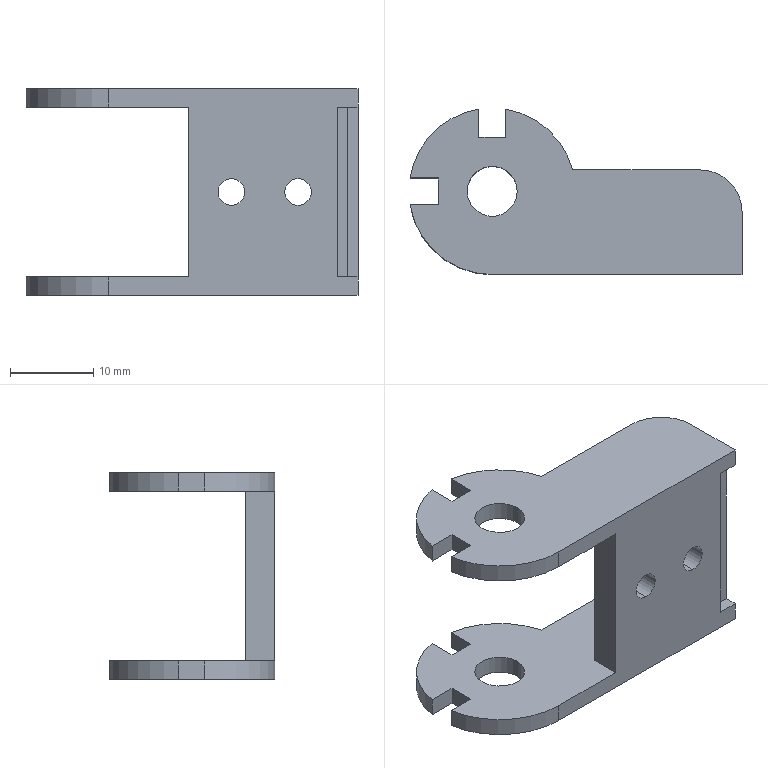Part | STEP file | TWD15-C15-R28-3_free | 1 solid | 48 faces | box 39.871 x 19.871 x 24.8 mm | volume 3618 mm3 | plane 28 | cylinder 16 | cone 4 | commonest cylinder face diameters 20 x6 3.2 x4 6 x4 10 x2
STEP:
#1=CARTESIAN_POINT('',(-15.2,2.5,-1.6));
#2=VERTEX_POINT('',#1);
#3=CARTESIAN_POINT('',(-15.2,2.5,1.6));
#4=VERTEX_POINT('',#3);
#5=CARTESIAN_POINT('',(-15.2,2.5,0.));
#6=DIRECTION('',(0.,-1.,0.));
#7=DIRECTION('',(0.,0.,1.));
#8=AXIS2_PLACEMENT_3D('',#5,#6,#7);
#9=CIRCLE('',#8,1.6);
#10=EDGE_CURVE('',#2,#4,#9,.T.);
#11=ORIENTED_EDGE('',*,*,#10,.F.);
#12=CARTESIAN_POINT('',(-15.2,0.,-1.6));
#13=VERTEX_POINT('',#12);
#14=CARTESIAN_POINT('',(-15.2,0.,-1.6));
#15=DIRECTION('',(0.,-1.,0.));
#16=VECTOR('',#15,1000.);
#17=LINE('',#14,#16);
#18=EDGE_CURVE('',#2,#13,#17,.T.);
#19=ORIENTED_EDGE('',*,*,#18,.T.);
#20=CARTESIAN_POINT('',(-15.2,0.,1.6));
#21=VERTEX_POINT('',#20);
#22=CARTESIAN_POINT('',(-15.2,0.,0.));
#23=DIRECTION('',(0.,-1.,0.));
#24=DIRECTION('',(0.,0.,-1.));
#25=AXIS2_PLACEMENT_3D('',#22,#23,#24);
#26=CIRCLE('',#25,1.6);
#27=EDGE_CURVE('',#13,#21,#26,.T.);
#28=ORIENTED_EDGE('',*,*,#27,.T.);
#29=CARTESIAN_POINT('',(-15.2,0.,1.6));
#30=DIRECTION('',(0.,-1.,0.));
#31=VECTOR('',#30,1000.);
#32=LINE('',#29,#31);
#33=EDGE_CURVE('',#4,#21,#32,.T.);
#34=ORIENTED_EDGE('',*,*,#33,.F.);
#35=EDGE_LOOP('',(#11,#19,#28,#34));
#36=FACE_OUTER_BOUND('',#35,.T.);
#37=CARTESIAN_POINT('',(-15.2,0.,0.));
#38=DIRECTION('',(0.,-1.,0.));
#39=DIRECTION('',(0.000000142,0.,1.));
#40=AXIS2_PLACEMENT_3D('',#37,#38,#39);
#41=CYLINDRICAL_SURFACE('',#40,1.6);
#42=ADVANCED_FACE('',(#36),#41,.F.);
#43=ORIENTED_EDGE('',*,*,#10,.T.);
#44=CARTESIAN_POINT('',(-15.2,3.5,2.6));
#45=VERTEX_POINT('',#44);
#46=CARTESIAN_POINT('',(-15.2,3.5,2.6));
#47=DIRECTION('',(0.,0.7071,0.7071));
#48=VECTOR('',#47,1000.);
#49=LINE('',#46,#48);
#50=EDGE_CURVE('',#4,#45,#49,.T.);
#51=ORIENTED_EDGE('',*,*,#50,.T.);
#52=CARTESIAN_POINT('',(-15.2,3.5,-2.6));
#53=VERTEX_POINT('',#52);
#54=CARTESIAN_POINT('',(-15.2,3.5,0.));
#55=DIRECTION('',(0.,-1.,0.));
#56=DIRECTION('',(0.,0.,1.));
#57=AXIS2_PLACEMENT_3D('',#54,#55,#56);
#58=CIRCLE('',#57,2.6);
#59=EDGE_CURVE('',#53,#45,#58,.T.);
#60=ORIENTED_EDGE('',*,*,#59,.F.);
#61=CARTESIAN_POINT('',(-15.2,3.5,-2.6));
#62=DIRECTION('',(0.,0.7071,-0.7071));
#63=VECTOR('',#62,1000.);
#64=LINE('',#61,#63);
#65=EDGE_CURVE('',#2,#53,#64,.T.);
#66=ORIENTED_EDGE('',*,*,#65,.F.);
#67=EDGE_LOOP('',(#43,#51,#60,#66));
#68=FACE_OUTER_BOUND('',#67,.T.);
#69=CARTESIAN_POINT('',(-15.2,3.5,0.));
#70=DIRECTION('',(0.,1.,0.));
#71=DIRECTION('',(0.,0.,-1.));
#72=AXIS2_PLACEMENT_3D('',#69,#70,#71);
#73=CONICAL_SURFACE('',#72,2.6,0.7854);
#74=ADVANCED_FACE('',(#68),#73,.F.);
#75=CARTESIAN_POINT('',(-7.2,2.5,-1.6));
#76=VERTEX_POINT('',#75);
#77=CARTESIAN_POINT('',(-7.2,2.5,1.6));
#78=VERTEX_POINT('',#77);
#79=CARTESIAN_POINT('',(-7.2,2.5,0.));
#80=DIRECTION('',(0.,-1.,0.));
#81=DIRECTION('',(0.,0.,1.));
#82=AXIS2_PLACEMENT_3D('',#79,#80,#81);
#83=CIRCLE('',#82,1.6);
#84=EDGE_CURVE('',#76,#78,#83,.T.);
#85=ORIENTED_EDGE('',*,*,#84,.F.);
#86=CARTESIAN_POINT('',(-7.2,0.,-1.6));
#87=VERTEX_POINT('',#86);
#88=CARTESIAN_POINT('',(-7.2,0.,-1.6));
#89=DIRECTION('',(0.,-1.,0.));
#90=VECTOR('',#89,1000.);
#91=LINE('',#88,#90);
#92=EDGE_CURVE('',#76,#87,#91,.T.);
#93=ORIENTED_EDGE('',*,*,#92,.T.);
#94=CARTESIAN_POINT('',(-7.2,0.,1.6));
#95=VERTEX_POINT('',#94);
#96=CARTESIAN_POINT('',(-7.2,0.,0.));
#97=DIRECTION('',(0.,-1.,0.));
#98=DIRECTION('',(0.,0.,-1.));
#99=AXIS2_PLACEMENT_3D('',#96,#97,#98);
#100=CIRCLE('',#99,1.6);
#101=EDGE_CURVE('',#87,#95,#100,.T.);
#102=ORIENTED_EDGE('',*,*,#101,.T.);
#103=CARTESIAN_POINT('',(-7.2,0.,1.6));
#104=DIRECTION('',(0.,-1.,0.));
#105=VECTOR('',#104,1000.);
#106=LINE('',#103,#105);
#107=EDGE_CURVE('',#78,#95,#106,.T.);
#108=ORIENTED_EDGE('',*,*,#107,.F.);
#109=EDGE_LOOP('',(#85,#93,#102,#108));
#110=FACE_OUTER_BOUND('',#109,.T.);
#111=CARTESIAN_POINT('',(-7.2,0.,0.));
#112=DIRECTION('',(0.,-1.,0.));
#113=DIRECTION('',(0.000000142,0.,1.));
#114=AXIS2_PLACEMENT_3D('',#111,#112,#113);
#115=CYLINDRICAL_SURFACE('',#114,1.6);
#116=ADVANCED_FACE('',(#110),#115,.F.);
#117=ORIENTED_EDGE('',*,*,#84,.T.);
#118=CARTESIAN_POINT('',(-7.2,3.5,2.6));
#119=VERTEX_POINT('',#118);
#120=CARTESIAN_POINT('',(-7.2,3.5,2.6));
#121=DIRECTION('',(0.,0.7071,0.7071));
#122=VECTOR('',#121,1000.);
#123=LINE('',#120,#122);
#124=EDGE_CURVE('',#78,#119,#123,.T.);
#125=ORIENTED_EDGE('',*,*,#124,.T.);
#126=CARTESIAN_POINT('',(-7.2,3.5,-2.6));
#127=VERTEX_POINT('',#126);
#128=CARTESIAN_POINT('',(-7.2,3.5,0.));
#129=DIRECTION('',(0.,-1.,0.));
#130=DIRECTION('',(-0.000000142,0.,1.));
#131=AXIS2_PLACEMENT_3D('',#128,#129,#130);
#132=CIRCLE('',#131,2.6);
#133=EDGE_CURVE('',#127,#119,#132,.T.);
#134=ORIENTED_EDGE('',*,*,#133,.F.);
#135=CARTESIAN_POINT('',(-7.2,3.5,-2.6));
#136=DIRECTION('',(0.,0.7071,-0.7071));
#137=VECTOR('',#136,1000.);
#138=LINE('',#135,#137);
#139=EDGE_CURVE('',#76,#127,#138,.T.);
#140=ORIENTED_EDGE('',*,*,#139,.F.);
#141=EDGE_LOOP('',(#117,#125,#134,#140));
#142=FACE_OUTER_BOUND('',#141,.T.);
#143=CARTESIAN_POINT('',(-7.2,3.5,0.));
#144=DIRECTION('',(0.,1.,0.));
#145=DIRECTION('',(0.,0.,-1.));
#146=AXIS2_PLACEMENT_3D('',#143,#144,#145);
#147=CONICAL_SURFACE('',#146,2.6,0.7854);
#148=ADVANCED_FACE('',(#142),#147,.F.);
#149=CARTESIAN_POINT('',(-27.,10.,12.4));
#150=VERTEX_POINT('',#149);
#151=CARTESIAN_POINT('',(-33.,10.,12.4));
#152=VERTEX_POINT('',#151);
#153=CARTESIAN_POINT('',(-30.,10.,12.4));
#154=DIRECTION('',(0.,0.,1.));
#155=DIRECTION('',(1.,0.,0.));
#156=AXIS2_PLACEMENT_3D('',#153,#154,#155);
#157=CIRCLE('',#156,3.);
#158=EDGE_CURVE('',#150,#152,#157,.T.);
#159=ORIENTED_EDGE('',*,*,#158,.T.);
#160=CARTESIAN_POINT('',(-33.,10.,10.2));
#161=VERTEX_POINT('',#160);
#162=CARTESIAN_POINT('',(-33.,10.,12.4));
#163=DIRECTION('',(0.,0.,-1.));
#164=VECTOR('',#163,1000.);
#165=LINE('',#162,#164);
#166=EDGE_CURVE('',#152,#161,#165,.T.);
#167=ORIENTED_EDGE('',*,*,#166,.T.);
#168=CARTESIAN_POINT('',(-27.,10.,10.2));
#169=VERTEX_POINT('',#168);
#170=CARTESIAN_POINT('',(-30.,10.,10.2));
#171=DIRECTION('',(0.,0.,1.));
#172=DIRECTION('',(-1.,0.,0.));
#173=AXIS2_PLACEMENT_3D('',#170,#171,#172);
#174=CIRCLE('',#173,3.);
#175=EDGE_CURVE('',#169,#161,#174,.T.);
#176=ORIENTED_EDGE('',*,*,#175,.F.);
#177=CARTESIAN_POINT('',(-27.,10.,12.4));
#178=DIRECTION('',(0.,0.,-1.));
#179=VECTOR('',#178,1000.);
#180=LINE('',#177,#179);
#181=EDGE_CURVE('',#150,#169,#180,.T.);
#182=ORIENTED_EDGE('',*,*,#181,.F.);
#183=EDGE_LOOP('',(#159,#167,#176,#182));
#184=FACE_OUTER_BOUND('',#183,.T.);
#185=CARTESIAN_POINT('',(-30.,10.,12.4));
#186=DIRECTION('',(0.,0.,-1.));
#187=DIRECTION('',(1.,0.,0.));
#188=AXIS2_PLACEMENT_3D('',#185,#186,#187);
#189=CYLINDRICAL_SURFACE('',#188,3.);
#190=ADVANCED_FACE('',(#184),#189,.F.);
#191=CARTESIAN_POINT('',(-27.,10.,-10.2));
#192=VERTEX_POINT('',#191);
#193=CARTESIAN_POINT('',(-33.,10.,-10.2));
#194=VERTEX_POINT('',#193);
#195=CARTESIAN_POINT('',(-30.,10.,-10.2));
#196=DIRECTION('',(0.,0.,1.));
#197=DIRECTION('',(1.,0.,0.));
#198=AXIS2_PLACEMENT_3D('',#195,#196,#197);
#199=CIRCLE('',#198,3.);
#200=EDGE_CURVE('',#192,#194,#199,.T.);
#201=ORIENTED_EDGE('',*,*,#200,.T.);
#202=CARTESIAN_POINT('',(-33.,10.,-12.4));
#203=VERTEX_POINT('',#202);
#204=CARTESIAN_POINT('',(-33.,10.,12.4));
#205=DIRECTION('',(0.,0.,-1.));
#206=VECTOR('',#205,1000.);
#207=LINE('',#204,#206);
#208=EDGE_CURVE('',#194,#203,#207,.T.);
#209=ORIENTED_EDGE('',*,*,#208,.T.);
#210=CARTESIAN_POINT('',(-27.,10.,-12.4));
#211=VERTEX_POINT('',#210);
#212=CARTESIAN_POINT('',(-30.,10.,-12.4));
#213=DIRECTION('',(0.,0.,1.));
#214=DIRECTION('',(-1.,0.,0.));
#215=AXIS2_PLACEMENT_3D('',#212,#213,#214);
#216=CIRCLE('',#215,3.);
#217=EDGE_CURVE('',#211,#203,#216,.T.);
#218=ORIENTED_EDGE('',*,*,#217,.F.);
#219=CARTESIAN_POINT('',(-27.,10.,12.4));
#220=DIRECTION('',(0.,0.,-1.));
#221=VECTOR('',#220,1000.);
#222=LINE('',#219,#221);
#223=EDGE_CURVE('',#192,#211,#222,.T.);
#224=ORIENTED_EDGE('',*,*,#223,.F.);
#225=EDGE_LOOP('',(#201,#209,#218,#224));
#226=FACE_OUTER_BOUND('',#225,.T.);
#227=CARTESIAN_POINT('',(-30.,10.,12.4));
#228=DIRECTION('',(0.,0.,-1.));
#229=DIRECTION('',(1.,0.,0.));
#230=AXIS2_PLACEMENT_3D('',#227,#228,#229);
#231=CYLINDRICAL_SURFACE('',#230,3.);
#232=ADVANCED_FACE('',(#226),#231,.F.);
#233=CARTESIAN_POINT('',(-31.6,19.871,-12.4));
#234=VERTEX_POINT('',#233);
#235=CARTESIAN_POINT('',(-31.6,19.871,-10.2));
#236=VERTEX_POINT('',#235);
#237=CARTESIAN_POINT('',(-31.6,19.871,-10.2));
#238=DIRECTION('',(0.,0.,1.));
#239=VECTOR('',#238,1000.);
#240=LINE('',#237,#239);
#241=EDGE_CURVE('',#234,#236,#240,.T.);
#242=ORIENTED_EDGE('',*,*,#241,.F.);
#243=CARTESIAN_POINT('',(-39.871,11.6,-12.4));
#244=VERTEX_POINT('',#243);
#245=CARTESIAN_POINT('',(-30.,10.,-12.4));
#246=DIRECTION('',(0.,0.,1.));
#247=DIRECTION('',(-0.16,0.9871,0.));
#248=AXIS2_PLACEMENT_3D('',#245,#246,#247);
#249=CIRCLE('',#248,10.);
#250=EDGE_CURVE('',#234,#244,#249,.T.);
#251=ORIENTED_EDGE('',*,*,#250,.T.);
#252=CARTESIAN_POINT('',(-39.871,11.6,-10.2));
#253=VERTEX_POINT('',#252);
#254=CARTESIAN_POINT('',(-39.871,11.6,-12.4));
#255=DIRECTION('',(0.,0.,-1.));
#256=VECTOR('',#255,1000.);
#257=LINE('',#254,#256);
#258=EDGE_CURVE('',#253,#244,#257,.T.);
#259=ORIENTED_EDGE('',*,*,#258,.F.);
#260=CARTESIAN_POINT('',(-30.,10.,-10.2));
#261=DIRECTION('',(0.,0.,1.));
#262=DIRECTION('',(-0.9871,0.16,0.));
#263=AXIS2_PLACEMENT_3D('',#260,#261,#262);
#264=CIRCLE('',#263,10.);
#265=EDGE_CURVE('',#236,#253,#264,.T.);
#266=ORIENTED_EDGE('',*,*,#265,.F.);
#267=EDGE_LOOP('',(#242,#251,#259,#266));
#268=FACE_OUTER_BOUND('',#267,.T.);
#269=CARTESIAN_POINT('',(-30.,10.,12.4));
#270=DIRECTION('',(0.,0.,-1.));
#271=DIRECTION('',(-0.9871,0.16,0.));
#272=AXIS2_PLACEMENT_3D('',#269,#270,#271);
#273=CYLINDRICAL_SURFACE('',#272,10.);
#274=ADVANCED_FACE('',(#268),#273,.T.);
#275=CARTESIAN_POINT('',(-28.4,19.871,-10.2));
#276=VERTEX_POINT('',#275);
#277=CARTESIAN_POINT('',(-28.4,19.871,-12.4));
#278=VERTEX_POINT('',#277);
#279=CARTESIAN_POINT('',(-28.4,19.871,-12.4));
#280=DIRECTION('',(0.,0.,-1.));
#281=VECTOR('',#280,1000.);
#282=LINE('',#279,#281);
#283=EDGE_CURVE('',#276,#278,#282,.T.);
#284=ORIENTED_EDGE('',*,*,#283,.F.);
#285=CARTESIAN_POINT('',(-20.333,12.56,-10.2));
#286=VERTEX_POINT('',#285);
#287=CARTESIAN_POINT('',(-30.,10.,-10.2));
#288=DIRECTION('',(0.,0.,1.));
#289=DIRECTION('',(0.16,0.9871,0.));
#290=AXIS2_PLACEMENT_3D('',#287,#288,#289);
#291=CIRCLE('',#290,10.);
#292=EDGE_CURVE('',#286,#276,#291,.T.);
#293=ORIENTED_EDGE('',*,*,#292,.F.);
#294=CARTESIAN_POINT('',(-20.333,12.56,-12.4));
#295=VERTEX_POINT('',#294);
#296=CARTESIAN_POINT('',(-20.333,12.56,-10.2));
#297=DIRECTION('',(0.,0.,-1.));
#298=VECTOR('',#297,1000.);
#299=LINE('',#296,#298);
#300=EDGE_CURVE('',#286,#295,#299,.T.);
#301=ORIENTED_EDGE('',*,*,#300,.T.);
#302=CARTESIAN_POINT('',(-30.,10.,-12.4));
#303=DIRECTION('',(0.,0.,1.));
#304=DIRECTION('',(0.9667,0.256,0.));
#305=AXIS2_PLACEMENT_3D('',#302,#303,#304);
#306=CIRCLE('',#305,10.);
#307=EDGE_CURVE('',#295,#278,#306,.T.);
#308=ORIENTED_EDGE('',*,*,#307,.T.);
#309=EDGE_LOOP('',(#284,#293,#301,#308));
#310=FACE_OUTER_BOUND('',#309,.T.);
#311=CARTESIAN_POINT('',(-30.,10.,12.4));
#312=DIRECTION('',(0.,0.,-1.));
#313=DIRECTION('',(0.16,0.9871,0.));
#314=AXIS2_PLACEMENT_3D('',#311,#312,#313);
#315=CYLINDRICAL_SURFACE('',#314,10.);
#316=ADVANCED_FACE('',(#310),#315,.T.);
#317=CARTESIAN_POINT('',(-31.6,19.871,10.2));
#318=VERTEX_POINT('',#317);
#319=CARTESIAN_POINT('',(-31.6,19.871,12.4));
#320=VERTEX_POINT('',#319);
#321=CARTESIAN_POINT('',(-31.6,19.871,12.4));
#322=DIRECTION('',(0.,0.,1.));
#323=VECTOR('',#322,1000.);
#324=LINE('',#321,#323);
#325=EDGE_CURVE('',#318,#320,#324,.T.);
#326=ORIENTED_EDGE('',*,*,#325,.F.);
#327=CARTESIAN_POINT('',(-39.871,11.6,10.2));
#328=VERTEX_POINT('',#327);
#329=CARTESIAN_POINT('',(-30.,10.,10.2));
#330=DIRECTION('',(0.,0.,1.));
#331=DIRECTION('',(-0.16,0.9871,0.));
#332=AXIS2_PLACEMENT_3D('',#329,#330,#331);
#333=CIRCLE('',#332,10.);
#334=EDGE_CURVE('',#318,#328,#333,.T.);
#335=ORIENTED_EDGE('',*,*,#334,.T.);
#336=CARTESIAN_POINT('',(-39.871,11.6,12.4));
#337=VERTEX_POINT('',#336);
#338=CARTESIAN_POINT('',(-39.871,11.6,10.2));
#339=DIRECTION('',(0.,0.,-1.));
#340=VECTOR('',#339,1000.);
#341=LINE('',#338,#340);
#342=EDGE_CURVE('',#337,#328,#341,.T.);
#343=ORIENTED_EDGE('',*,*,#342,.F.);
#344=CARTESIAN_POINT('',(-30.,10.,12.4));
#345=DIRECTION('',(0.,0.,1.));
#346=DIRECTION('',(-0.9871,0.16,0.));
#347=AXIS2_PLACEMENT_3D('',#344,#345,#346);
#348=CIRCLE('',#347,10.);
#349=EDGE_CURVE('',#320,#337,#348,.T.);
#350=ORIENTED_EDGE('',*,*,#349,.F.);
#351=EDGE_LOOP('',(#326,#335,#343,#350));
#352=FACE_OUTER_BOUND('',#351,.T.);
#353=CARTESIAN_POINT('',(-30.,10.,12.4));
#354=DIRECTION('',(0.,0.,-1.));
#355=DIRECTION('',(-0.9871,0.16,0.));
#356=AXIS2_PLACEMENT_3D('',#353,#354,#355);
#357=CYLINDRICAL_SURFACE('',#356,10.);
#358=ADVANCED_FACE('',(#352),#357,.T.);
#359=CARTESIAN_POINT('',(-28.4,19.871,12.4));
#360=VERTEX_POINT('',#359);
#361=CARTESIAN_POINT('',(-28.4,19.871,10.2));
#362=VERTEX_POINT('',#361);
#363=CARTESIAN_POINT('',(-28.4,19.871,10.2));
#364=DIRECTION('',(0.,0.,-1.));
#365=VECTOR('',#364,1000.);
#366=LINE('',#363,#365);
#367=EDGE_CURVE('',#360,#362,#366,.T.);
#368=ORIENTED_EDGE('',*,*,#367,.F.);
#369=CARTESIAN_POINT('',(-20.333,12.56,12.4));
#370=VERTEX_POINT('',#369);
#371=CARTESIAN_POINT('',(-30.,10.,12.4));
#372=DIRECTION('',(0.,0.,1.));
#373=DIRECTION('',(0.16,0.9871,0.));
#374=AXIS2_PLACEMENT_3D('',#371,#372,#373);
#375=CIRCLE('',#374,10.);
#376=EDGE_CURVE('',#370,#360,#375,.T.);
#377=ORIENTED_EDGE('',*,*,#376,.F.);
#378=CARTESIAN_POINT('',(-20.333,12.56,10.2));
#379=VERTEX_POINT('',#378);
#380=CARTESIAN_POINT('',(-20.333,12.56,12.4));
#381=DIRECTION('',(0.,0.,-1.));
#382=VECTOR('',#381,1000.);
#383=LINE('',#380,#382);
#384=EDGE_CURVE('',#370,#379,#383,.T.);
#385=ORIENTED_EDGE('',*,*,#384,.T.);
#386=CARTESIAN_POINT('',(-30.,10.,10.2));
#387=DIRECTION('',(0.,0.,1.));
#388=DIRECTION('',(0.9667,0.256,0.));
#389=AXIS2_PLACEMENT_3D('',#386,#387,#388);
#390=CIRCLE('',#389,10.);
#391=EDGE_CURVE('',#379,#362,#390,.T.);
#392=ORIENTED_EDGE('',*,*,#391,.T.);
#393=EDGE_LOOP('',(#368,#377,#385,#392));
#394=FACE_OUTER_BOUND('',#393,.T.);
#395=CARTESIAN_POINT('',(-30.,10.,12.4));
#396=DIRECTION('',(0.,0.,-1.));
#397=DIRECTION('',(0.16,0.9871,0.));
#398=AXIS2_PLACEMENT_3D('',#395,#396,#397);
#399=CYLINDRICAL_SURFACE('',#398,10.);
#400=ADVANCED_FACE('',(#394),#399,.T.);
#401=CARTESIAN_POINT('',(-31.6,16.5,12.4));
#402=VERTEX_POINT('',#401);
#403=CARTESIAN_POINT('',(-28.4,16.5,12.4));
#404=VERTEX_POINT('',#403);
#405=CARTESIAN_POINT('',(-28.4,16.5,12.4));
#406=DIRECTION('',(1.,0.,0.));
#407=VECTOR('',#406,1000.);
#408=LINE('',#405,#407);
#409=EDGE_CURVE('',#402,#404,#408,.T.);
#410=ORIENTED_EDGE('',*,*,#409,.F.);
#411=CARTESIAN_POINT('',(-31.6,16.5,12.4));
#412=DIRECTION('',(0.,-1.,0.));
#413=VECTOR('',#412,1000.);
#414=LINE('',#411,#413);
#415=EDGE_CURVE('',#320,#402,#414,.T.);
#416=ORIENTED_EDGE('',*,*,#415,.F.);
#417=ORIENTED_EDGE('',*,*,#349,.T.);
#418=CARTESIAN_POINT('',(-36.5,11.6,12.4));
#419=VERTEX_POINT('',#418);
#420=CARTESIAN_POINT('',(-39.871,11.6,12.4));
#421=DIRECTION('',(-1.,0.,0.));
#422=VECTOR('',#421,1000.);
#423=LINE('',#420,#422);
#424=EDGE_CURVE('',#419,#337,#423,.T.);
#425=ORIENTED_EDGE('',*,*,#424,.F.);
#426=CARTESIAN_POINT('',(-36.5,8.4,12.4));
#427=VERTEX_POINT('',#426);
#428=CARTESIAN_POINT('',(-36.5,11.6,12.4));
#429=DIRECTION('',(0.,1.,0.));
#430=VECTOR('',#429,1000.);
#431=LINE('',#428,#430);
#432=EDGE_CURVE('',#427,#419,#431,.T.);
#433=ORIENTED_EDGE('',*,*,#432,.F.);
#434=CARTESIAN_POINT('',(-39.871,8.4,12.4));
#435=VERTEX_POINT('',#434);
#436=CARTESIAN_POINT('',(-36.5,8.4,12.4));
#437=DIRECTION('',(1.,0.,0.));
#438=VECTOR('',#437,1000.);
#439=LINE('',#436,#438);
#440=EDGE_CURVE('',#435,#427,#439,.T.);
#441=ORIENTED_EDGE('',*,*,#440,.F.);
#442=CARTESIAN_POINT('',(-30.,0.,12.4));
#443=VERTEX_POINT('',#442);
#444=CARTESIAN_POINT('',(-30.,10.,12.4));
#445=DIRECTION('',(0.,0.,1.));
#446=DIRECTION('',(-0.9871,-0.16,0.));
#447=AXIS2_PLACEMENT_3D('',#444,#445,#446);
#448=CIRCLE('',#447,10.);
#449=EDGE_CURVE('',#435,#443,#448,.T.);
#450=ORIENTED_EDGE('',*,*,#449,.T.);
#451=CARTESIAN_POINT('',(0.,0.,12.4));
#452=VERTEX_POINT('',#451);
#453=CARTESIAN_POINT('',(-30.,0.,12.4));
#454=DIRECTION('',(1.,0.,0.));
#455=VECTOR('',#454,1000.);
#456=LINE('',#453,#455);
#457=EDGE_CURVE('',#443,#452,#456,.T.);
#458=ORIENTED_EDGE('',*,*,#457,.T.);
#459=CARTESIAN_POINT('',(0.,7.56,12.4));
#460=VERTEX_POINT('',#459);
#461=CARTESIAN_POINT('',(0.,0.,12.4));
#462=DIRECTION('',(0.,1.,0.));
#463=VECTOR('',#462,1000.);
#464=LINE('',#461,#463);
#465=EDGE_CURVE('',#452,#460,#464,.T.);
#466=ORIENTED_EDGE('',*,*,#465,.T.);
#467=CARTESIAN_POINT('',(-5.,12.56,12.4));
#468=VERTEX_POINT('',#467);
#469=CARTESIAN_POINT('',(-5.,7.56,12.4));
#470=DIRECTION('',(0.,0.,1.));
#471=DIRECTION('',(1.,0.,0.));
#472=AXIS2_PLACEMENT_3D('',#469,#470,#471);
#473=CIRCLE('',#472,5.);
#474=EDGE_CURVE('',#460,#468,#473,.T.);
#475=ORIENTED_EDGE('',*,*,#474,.T.);
#476=CARTESIAN_POINT('',(-5.,12.56,12.4));
#477=DIRECTION('',(-1.,0.,0.));
#478=VECTOR('',#477,1000.);
#479=LINE('',#476,#478);
#480=EDGE_CURVE('',#468,#370,#479,.T.);
#481=ORIENTED_EDGE('',*,*,#480,.T.);
#482=ORIENTED_EDGE('',*,*,#376,.T.);
#483=CARTESIAN_POINT('',(-28.4,19.871,12.4));
#484=DIRECTION('',(0.,1.,0.));
#485=VECTOR('',#484,1000.);
#486=LINE('',#483,#485);
#487=EDGE_CURVE('',#404,#360,#486,.T.);
#488=ORIENTED_EDGE('',*,*,#487,.F.);
#489=EDGE_LOOP('',(#410,#416,#417,#425,#433,#441,#450,#458,#466,#475,#481,#482,#488));
#490=FACE_OUTER_BOUND('',#489,.T.);
#491=ORIENTED_EDGE('',*,*,#158,.F.);
#492=CARTESIAN_POINT('',(-30.,10.,12.4));
#493=DIRECTION('',(0.,0.,1.));
#494=DIRECTION('',(1.,0.,0.));
#495=AXIS2_PLACEMENT_3D('',#492,#493,#494);
#496=CIRCLE('',#495,3.);
#497=EDGE_CURVE('',#152,#150,#496,.T.);
#498=ORIENTED_EDGE('',*,*,#497,.F.);
#499=EDGE_LOOP('',(#491,#498));
#500=FACE_BOUND('',#499,.T.);
#501=CARTESIAN_POINT('',(-39.871,0.,12.4));
#502=DIRECTION('',(0.,0.,1.));
#503=DIRECTION('',(1.,0.,0.));
#504=AXIS2_PLACEMENT_3D('',#501,#502,#503);
#505=PLANE('',#504);
#506=ADVANCED_FACE('',(#490,#500),#505,.T.);
#507=CARTESIAN_POINT('',(-31.6,16.5,-12.4));
#508=VERTEX_POINT('',#507);
#509=CARTESIAN_POINT('',(-31.6,19.871,-12.4));
#510=DIRECTION('',(0.,-1.,0.));
#511=VECTOR('',#510,1000.);
#512=LINE('',#509,#511);
#513=EDGE_CURVE('',#234,#508,#512,.T.);
#514=ORIENTED_EDGE('',*,*,#513,.T.);
#515=CARTESIAN_POINT('',(-28.4,16.5,-12.4));
#516=VERTEX_POINT('',#515);
#517=CARTESIAN_POINT('',(-31.6,16.5,-12.4));
#518=DIRECTION('',(1.,0.,0.));
#519=VECTOR('',#518,1000.);
#520=LINE('',#517,#519);
#521=EDGE_CURVE('',#508,#516,#520,.T.);
#522=ORIENTED_EDGE('',*,*,#521,.T.);
#523=CARTESIAN_POINT('',(-28.4,16.5,-12.4));
#524=DIRECTION('',(0.,1.,0.));
#525=VECTOR('',#524,1000.);
#526=LINE('',#523,#525);
#527=EDGE_CURVE('',#516,#278,#526,.T.);
#528=ORIENTED_EDGE('',*,*,#527,.T.);
#529=ORIENTED_EDGE('',*,*,#307,.F.);
#530=CARTESIAN_POINT('',(-5.,12.56,-12.4));
#531=VERTEX_POINT('',#530);
#532=CARTESIAN_POINT('',(-20.333,12.56,-12.4));
#533=DIRECTION('',(-1.,0.,0.));
#534=VECTOR('',#533,1000.);
#535=LINE('',#532,#534);
#536=EDGE_CURVE('',#531,#295,#535,.T.);
#537=ORIENTED_EDGE('',*,*,#536,.F.);
#538=CARTESIAN_POINT('',(0.,7.56,-12.4));
#539=VERTEX_POINT('',#538);
#540=CARTESIAN_POINT('',(-5.,7.56,-12.4));
#541=DIRECTION('',(0.,0.,1.));
#542=DIRECTION('',(0.,1.,0.));
#543=AXIS2_PLACEMENT_3D('',#540,#541,#542);
#544=CIRCLE('',#543,5.);
#545=EDGE_CURVE('',#539,#531,#544,.T.);
#546=ORIENTED_EDGE('',*,*,#545,.F.);
#547=CARTESIAN_POINT('',(0.,0.,-12.4));
#548=VERTEX_POINT('',#547);
#549=CARTESIAN_POINT('',(0.,7.56,-12.4));
#550=DIRECTION('',(0.,1.,0.));
#551=VECTOR('',#550,1000.);
#552=LINE('',#549,#551);
#553=EDGE_CURVE('',#548,#539,#552,.T.);
#554=ORIENTED_EDGE('',*,*,#553,.F.);
#555=CARTESIAN_POINT('',(-30.,0.,-12.4));
#556=VERTEX_POINT('',#555);
#557=CARTESIAN_POINT('',(0.,0.,-12.4));
#558=DIRECTION('',(1.,0.,0.));
#559=VECTOR('',#558,1000.);
#560=LINE('',#557,#559);
#561=EDGE_CURVE('',#556,#548,#560,.T.);
#562=ORIENTED_EDGE('',*,*,#561,.F.);
#563=CARTESIAN_POINT('',(-39.871,8.4,-12.4));
#564=VERTEX_POINT('',#563);
#565=CARTESIAN_POINT('',(-30.,10.,-12.4));
#566=DIRECTION('',(0.,0.,1.));
#567=DIRECTION('',(0.,-1.,0.));
#568=AXIS2_PLACEMENT_3D('',#565,#566,#567);
#569=CIRCLE('',#568,10.);
#570=EDGE_CURVE('',#564,#556,#569,.T.);
#571=ORIENTED_EDGE('',*,*,#570,.F.);
#572=CARTESIAN_POINT('',(-36.5,8.4,-12.4));
#573=VERTEX_POINT('',#572);
#574=CARTESIAN_POINT('',(-39.871,8.4,-12.4));
#575=DIRECTION('',(1.,0.,0.));
#576=VECTOR('',#575,1000.);
#577=LINE('',#574,#576);
#578=EDGE_CURVE('',#564,#573,#577,.T.);
#579=ORIENTED_EDGE('',*,*,#578,.T.);
#580=CARTESIAN_POINT('',(-36.5,11.6,-12.4));
#581=VERTEX_POINT('',#580);
#582=CARTESIAN_POINT('',(-36.5,8.4,-12.4));
#583=DIRECTION('',(0.,1.,0.));
#584=VECTOR('',#583,1000.);
#585=LINE('',#582,#584);
#586=EDGE_CURVE('',#573,#581,#585,.T.);
#587=ORIENTED_EDGE('',*,*,#586,.T.);
#588=CARTESIAN_POINT('',(-36.5,11.6,-12.4));
#589=DIRECTION('',(-1.,0.,0.));
#590=VECTOR('',#589,1000.);
#591=LINE('',#588,#590);
#592=EDGE_CURVE('',#581,#244,#591,.T.);
#593=ORIENTED_EDGE('',*,*,#592,.T.);
#594=ORIENTED_EDGE('',*,*,#250,.F.);
#595=EDGE_LOOP('',(#514,#522,#528,#529,#537,#546,#554,#562,#571,#579,#587,#593,#594));
#596=FACE_OUTER_BOUND('',#595,.T.);
#597=ORIENTED_EDGE('',*,*,#217,.T.);
#598=CARTESIAN_POINT('',(-30.,10.,-12.4));
#599=DIRECTION('',(0.,0.,1.));
#600=DIRECTION('',(-1.,0.,0.));
#601=AXIS2_PLACEMENT_3D('',#598,#599,#600);
#602=CIRCLE('',#601,3.);
#603=EDGE_CURVE('',#203,#211,#602,.T.);
#604=ORIENTED_EDGE('',*,*,#603,.T.);
#605=EDGE_LOOP('',(#597,#604));
#606=FACE_BOUND('',#605,.T.);
#607=CARTESIAN_POINT('',(-39.871,0.,-12.4));
#608=DIRECTION('',(0.,0.,-1.));
#609=DIRECTION('',(0.,1.,0.));
#610=AXIS2_PLACEMENT_3D('',#607,#608,#609);
#611=PLANE('',#610);
#612=ADVANCED_FACE('',(#596,#606),#611,.T.);
#613=CARTESIAN_POINT('',(-31.6,16.5,10.2));
#614=VERTEX_POINT('',#613);
#615=CARTESIAN_POINT('',(-31.6,19.871,10.2));
#616=DIRECTION('',(0.,1.,0.));
#617=VECTOR('',#616,1000.);
#618=LINE('',#615,#617);
#619=EDGE_CURVE('',#614,#318,#618,.T.);
#620=ORIENTED_EDGE('',*,*,#619,.F.);
#621=CARTESIAN_POINT('',(-28.4,16.5,10.2));
#622=VERTEX_POINT('',#621);
#623=CARTESIAN_POINT('',(-31.6,16.5,10.2));
#624=DIRECTION('',(-1.,0.,0.));
#625=VECTOR('',#624,1000.);
#626=LINE('',#623,#625);
#627=EDGE_CURVE('',#622,#614,#626,.T.);
#628=ORIENTED_EDGE('',*,*,#627,.F.);
#629=CARTESIAN_POINT('',(-28.4,16.5,10.2));
#630=DIRECTION('',(0.,-1.,0.));
#631=VECTOR('',#630,1000.);
#632=LINE('',#629,#631);
#633=EDGE_CURVE('',#362,#622,#632,.T.);
#634=ORIENTED_EDGE('',*,*,#633,.F.);
#635=ORIENTED_EDGE('',*,*,#391,.F.);
#636=CARTESIAN_POINT('',(-5.,12.56,10.2));
#637=VERTEX_POINT('',#636);
#638=CARTESIAN_POINT('',(-20.333,12.56,10.2));
#639=DIRECTION('',(-1.,0.,0.));
#640=VECTOR('',#639,1000.);
#641=LINE('',#638,#640);
#642=EDGE_CURVE('',#637,#379,#641,.T.);
#643=ORIENTED_EDGE('',*,*,#642,.F.);
#644=CARTESIAN_POINT('',(0.,7.56,10.2));
#645=VERTEX_POINT('',#644);
#646=CARTESIAN_POINT('',(-5.,7.56,10.2));
#647=DIRECTION('',(0.,0.,1.));
#648=DIRECTION('',(0.,1.,0.));
#649=AXIS2_PLACEMENT_3D('',#646,#647,#648);
#650=CIRCLE('',#649,5.);
#651=EDGE_CURVE('',#645,#637,#650,.T.);
#652=ORIENTED_EDGE('',*,*,#651,.F.);
#653=CARTESIAN_POINT('',(0.,3.5,10.2));
#654=VERTEX_POINT('',#653);
#655=CARTESIAN_POINT('',(0.,7.56,10.2));
#656=DIRECTION('',(0.,1.,0.));
#657=VECTOR('',#656,1000.);
#658=LINE('',#655,#657);
#659=EDGE_CURVE('',#654,#645,#658,.T.);
#660=ORIENTED_EDGE('',*,*,#659,.F.);
#661=CARTESIAN_POINT('',(-20.32,3.5,10.2));
#662=VERTEX_POINT('',#661);
#663=CARTESIAN_POINT('',(0.,3.5,10.2));
#664=DIRECTION('',(-1.,0.,0.));
#665=VECTOR('',#664,1000.);
#666=LINE('',#663,#665);
#667=EDGE_CURVE('',#654,#662,#666,.T.);
#668=ORIENTED_EDGE('',*,*,#667,.T.);
#669=CARTESIAN_POINT('',(-20.32,0.,10.2));
#670=VERTEX_POINT('',#669);
#671=CARTESIAN_POINT('',(-20.32,3.5,10.2));
#672=DIRECTION('',(0.,-1.,0.));
#673=VECTOR('',#672,1000.);
#674=LINE('',#671,#673);
#675=EDGE_CURVE('',#662,#670,#674,.T.);
#676=ORIENTED_EDGE('',*,*,#675,.T.);
#677=CARTESIAN_POINT('',(-30.,0.,10.2));
#678=VERTEX_POINT('',#677);
#679=CARTESIAN_POINT('',(-20.32,0.,10.2));
#680=DIRECTION('',(1.,0.,0.));
#681=VECTOR('',#680,1000.);
#682=LINE('',#679,#681);
#683=EDGE_CURVE('',#678,#670,#682,.T.);
#684=ORIENTED_EDGE('',*,*,#683,.F.);
#685=CARTESIAN_POINT('',(-39.871,8.4,10.2));
#686=VERTEX_POINT('',#685);
#687=CARTESIAN_POINT('',(-30.,10.,10.2));
#688=DIRECTION('',(0.,0.,1.));
#689=DIRECTION('',(0.,-1.,0.));
#690=AXIS2_PLACEMENT_3D('',#687,#688,#689);
#691=CIRCLE('',#690,10.);
#692=EDGE_CURVE('',#686,#678,#691,.T.);
#693=ORIENTED_EDGE('',*,*,#692,.F.);
#694=CARTESIAN_POINT('',(-36.5,8.4,10.2));
#695=VERTEX_POINT('',#694);
#696=CARTESIAN_POINT('',(-39.871,8.4,10.2));
#697=DIRECTION('',(-1.,0.,0.));
#698=VECTOR('',#697,1000.);
#699=LINE('',#696,#698);
#700=EDGE_CURVE('',#695,#686,#699,.T.);
#701=ORIENTED_EDGE('',*,*,#700,.F.);
#702=CARTESIAN_POINT('',(-36.5,11.6,10.2));
#703=VERTEX_POINT('',#702);
#704=CARTESIAN_POINT('',(-36.5,8.4,10.2));
#705=DIRECTION('',(0.,-1.,0.));
#706=VECTOR('',#705,1000.);
#707=LINE('',#704,#706);
#708=EDGE_CURVE('',#703,#695,#707,.T.);
#709=ORIENTED_EDGE('',*,*,#708,.F.);
#710=CARTESIAN_POINT('',(-36.5,11.6,10.2));
#711=DIRECTION('',(1.,0.,0.));
#712=VECTOR('',#711,1000.);
#713=LINE('',#710,#712);
#714=EDGE_CURVE('',#328,#703,#713,.T.);
#715=ORIENTED_EDGE('',*,*,#714,.F.);
#716=ORIENTED_EDGE('',*,*,#334,.F.);
#717=EDGE_LOOP('',(#620,#628,#634,#635,#643,#652,#660,#668,#676,#684,#693,#701,#709,#715,#716));
#718=FACE_OUTER_BOUND('',#717,.T.);
#719=ORIENTED_EDGE('',*,*,#175,.T.);
#720=CARTESIAN_POINT('',(-30.,10.,10.2));
#721=DIRECTION('',(0.,0.,1.));
#722=DIRECTION('',(-1.,0.,0.));
#723=AXIS2_PLACEMENT_3D('',#720,#721,#722);
#724=CIRCLE('',#723,3.);
#725=EDGE_CURVE('',#161,#169,#724,.T.);
#726=ORIENTED_EDGE('',*,*,#725,.T.);
#727=EDGE_LOOP('',(#719,#726));
#728=FACE_BOUND('',#727,.T.);
#729=CARTESIAN_POINT('',(-39.871,0.,10.2));
#730=DIRECTION('',(0.,0.,-1.));
#731=DIRECTION('',(0.,1.,0.));
#732=AXIS2_PLACEMENT_3D('',#729,#730,#731);
#733=PLANE('',#732);
#734=ADVANCED_FACE('',(#718,#728),#733,.T.);
#735=CARTESIAN_POINT('',(-28.4,16.5,-10.2));
#736=VERTEX_POINT('',#735);
#737=CARTESIAN_POINT('',(-31.6,16.5,-10.2));
#738=VERTEX_POINT('',#737);
#739=CARTESIAN_POINT('',(-28.4,16.5,-10.2));
#740=DIRECTION('',(-1.,0.,0.));
#741=VECTOR('',#740,1000.);
#742=LINE('',#739,#741);
#743=EDGE_CURVE('',#736,#738,#742,.T.);
#744=ORIENTED_EDGE('',*,*,#743,.T.);
#745=CARTESIAN_POINT('',(-31.6,16.5,-10.2));
#746=DIRECTION('',(0.,1.,0.));
#747=VECTOR('',#746,1000.);
#748=LINE('',#745,#747);
#749=EDGE_CURVE('',#738,#236,#748,.T.);
#750=ORIENTED_EDGE('',*,*,#749,.T.);
#751=ORIENTED_EDGE('',*,*,#265,.T.);
#752=CARTESIAN_POINT('',(-36.5,11.6,-10.2));
#753=VERTEX_POINT('',#752);
#754=CARTESIAN_POINT('',(-39.871,11.6,-10.2));
#755=DIRECTION('',(1.,0.,0.));
#756=VECTOR('',#755,1000.);
#757=LINE('',#754,#756);
#758=EDGE_CURVE('',#253,#753,#757,.T.);
#759=ORIENTED_EDGE('',*,*,#758,.T.);
#760=CARTESIAN_POINT('',(-36.5,8.4,-10.2));
#761=VERTEX_POINT('',#760);
#762=CARTESIAN_POINT('',(-36.5,11.6,-10.2));
#763=DIRECTION('',(0.,-1.,0.));
#764=VECTOR('',#763,1000.);
#765=LINE('',#762,#764);
#766=EDGE_CURVE('',#753,#761,#765,.T.);
#767=ORIENTED_EDGE('',*,*,#766,.T.);
#768=CARTESIAN_POINT('',(-39.871,8.4,-10.2));
#769=VERTEX_POINT('',#768);
#770=CARTESIAN_POINT('',(-36.5,8.4,-10.2));
#771=DIRECTION('',(-1.,0.,0.));
#772=VECTOR('',#771,1000.);
#773=LINE('',#770,#772);
#774=EDGE_CURVE('',#761,#769,#773,.T.);
#775=ORIENTED_EDGE('',*,*,#774,.T.);
#776=CARTESIAN_POINT('',(-30.,0.,-10.2));
#777=VERTEX_POINT('',#776);
#778=CARTESIAN_POINT('',(-30.,10.,-10.2));
#779=DIRECTION('',(0.,0.,1.));
#780=DIRECTION('',(-0.9871,-0.16,0.));
#781=AXIS2_PLACEMENT_3D('',#778,#779,#780);
#782=CIRCLE('',#781,10.);
#783=EDGE_CURVE('',#769,#777,#782,.T.);
#784=ORIENTED_EDGE('',*,*,#783,.T.);
#785=CARTESIAN_POINT('',(-20.32,0.,-10.2));
#786=VERTEX_POINT('',#785);
#787=CARTESIAN_POINT('',(-30.,0.,-10.2));
#788=DIRECTION('',(1.,0.,0.));
#789=VECTOR('',#788,1000.);
#790=LINE('',#787,#789);
#791=EDGE_CURVE('',#777,#786,#790,.T.);
#792=ORIENTED_EDGE('',*,*,#791,.T.);
#793=CARTESIAN_POINT('',(-20.32,3.5,-10.2));
#794=VERTEX_POINT('',#793);
#795=CARTESIAN_POINT('',(-20.32,0.,-10.2));
#796=DIRECTION('',(0.,-1.,0.));
#797=VECTOR('',#796,1000.);
#798=LINE('',#795,#797);
#799=EDGE_CURVE('',#794,#786,#798,.T.);
#800=ORIENTED_EDGE('',*,*,#799,.F.);
#801=CARTESIAN_POINT('',(0.,3.5,-10.2));
#802=VERTEX_POINT('',#801);
#803=CARTESIAN_POINT('',(-20.32,3.5,-10.2));
#804=DIRECTION('',(-1.,0.,0.));
#805=VECTOR('',#804,1000.);
#806=LINE('',#803,#805);
#807=EDGE_CURVE('',#802,#794,#806,.T.);
#808=ORIENTED_EDGE('',*,*,#807,.F.);
#809=CARTESIAN_POINT('',(0.,7.56,-10.2));
#810=VERTEX_POINT('',#809);
#811=CARTESIAN_POINT('',(0.,3.5,-10.2));
#812=DIRECTION('',(0.,1.,0.));
#813=VECTOR('',#812,1000.);
#814=LINE('',#811,#813);
#815=EDGE_CURVE('',#802,#810,#814,.T.);
#816=ORIENTED_EDGE('',*,*,#815,.T.);
#817=CARTESIAN_POINT('',(-5.,12.56,-10.2));
#818=VERTEX_POINT('',#817);
#819=CARTESIAN_POINT('',(-5.,7.56,-10.2));
#820=DIRECTION('',(0.,0.,1.));
#821=DIRECTION('',(1.,0.,0.));
#822=AXIS2_PLACEMENT_3D('',#819,#820,#821);
#823=CIRCLE('',#822,5.);
#824=EDGE_CURVE('',#810,#818,#823,.T.);
#825=ORIENTED_EDGE('',*,*,#824,.T.);
#826=CARTESIAN_POINT('',(-5.,12.56,-10.2));
#827=DIRECTION('',(-1.,0.,0.));
#828=VECTOR('',#827,1000.);
#829=LINE('',#826,#828);
#830=EDGE_CURVE('',#818,#286,#829,.T.);
#831=ORIENTED_EDGE('',*,*,#830,.T.);
#832=ORIENTED_EDGE('',*,*,#292,.T.);
#833=CARTESIAN_POINT('',(-28.4,19.871,-10.2));
#834=DIRECTION('',(0.,-1.,0.));
#835=VECTOR('',#834,1000.);
#836=LINE('',#833,#835);
#837=EDGE_CURVE('',#276,#736,#836,.T.);
#838=ORIENTED_EDGE('',*,*,#837,.T.);
#839=EDGE_LOOP('',(#744,#750,#751,#759,#767,#775,#784,#792,#800,#808,#816,#825,#831,#832,#838));
#840=FACE_OUTER_BOUND('',#839,.T.);
#841=ORIENTED_EDGE('',*,*,#200,.F.);
#842=CARTESIAN_POINT('',(-30.,10.,-10.2));
#843=DIRECTION('',(0.,0.,1.));
#844=DIRECTION('',(1.,0.,0.));
#845=AXIS2_PLACEMENT_3D('',#842,#843,#844);
#846=CIRCLE('',#845,3.);
#847=EDGE_CURVE('',#194,#192,#846,.T.);
#848=ORIENTED_EDGE('',*,*,#847,.F.);
#849=EDGE_LOOP('',(#841,#848));
#850=FACE_BOUND('',#849,.T.);
#851=CARTESIAN_POINT('',(-39.871,0.,-10.2));
#852=DIRECTION('',(0.,0.,1.));
#853=DIRECTION('',(1.,0.,0.));
#854=AXIS2_PLACEMENT_3D('',#851,#852,#853);
#855=PLANE('',#854);
#856=ADVANCED_FACE('',(#840,#850),#855,.T.);
#857=CARTESIAN_POINT('',(-39.871,8.4,-10.2));
#858=DIRECTION('',(0.,0.,1.));
#859=VECTOR('',#858,1000.);
#860=LINE('',#857,#859);
#861=EDGE_CURVE('',#564,#769,#860,.T.);
#862=ORIENTED_EDGE('',*,*,#861,.F.);
#863=ORIENTED_EDGE('',*,*,#570,.T.);
#864=CARTESIAN_POINT('',(-30.,0.,-12.4));
#865=DIRECTION('',(0.,0.,-1.));
#866=VECTOR('',#865,1000.);
#867=LINE('',#864,#866);
#868=EDGE_CURVE('',#777,#556,#867,.T.);
#869=ORIENTED_EDGE('',*,*,#868,.F.);
#870=ORIENTED_EDGE('',*,*,#783,.F.);
#871=EDGE_LOOP('',(#862,#863,#869,#870));
#872=FACE_OUTER_BOUND('',#871,.T.);
#873=CARTESIAN_POINT('',(-30.,10.,12.4));
#874=DIRECTION('',(0.,0.,-1.));
#875=DIRECTION('',(0.,-1.,0.));
#876=AXIS2_PLACEMENT_3D('',#873,#874,#875);
#877=CYLINDRICAL_SURFACE('',#876,10.);
#878=ADVANCED_FACE('',(#872),#877,.T.);
#879=CARTESIAN_POINT('',(-39.871,8.4,12.4));
#880=DIRECTION('',(0.,0.,1.));
#881=VECTOR('',#880,1000.);
#882=LINE('',#879,#881);
#883=EDGE_CURVE('',#686,#435,#882,.T.);
#884=ORIENTED_EDGE('',*,*,#883,.F.);
#885=ORIENTED_EDGE('',*,*,#692,.T.);
#886=CARTESIAN_POINT('',(-30.,0.,10.2));
#887=DIRECTION('',(0.,0.,-1.));
#888=VECTOR('',#887,1000.);
#889=LINE('',#886,#888);
#890=EDGE_CURVE('',#443,#678,#889,.T.);
#891=ORIENTED_EDGE('',*,*,#890,.F.);
#892=ORIENTED_EDGE('',*,*,#449,.F.);
#893=EDGE_LOOP('',(#884,#885,#891,#892));
#894=FACE_OUTER_BOUND('',#893,.T.);
#895=CARTESIAN_POINT('',(-30.,10.,12.4));
#896=DIRECTION('',(0.,0.,-1.));
#897=DIRECTION('',(0.,-1.,0.));
#898=AXIS2_PLACEMENT_3D('',#895,#896,#897);
#899=CYLINDRICAL_SURFACE('',#898,10.);
#900=ADVANCED_FACE('',(#894),#899,.T.);
#901=ORIENTED_EDGE('',*,*,#830,.F.);
#902=CARTESIAN_POINT('',(-5.,12.56,-10.2));
#903=DIRECTION('',(0.,0.,-1.));
#904=VECTOR('',#903,1000.);
#905=LINE('',#902,#904);
#906=EDGE_CURVE('',#818,#531,#905,.T.);
#907=ORIENTED_EDGE('',*,*,#906,.T.);
#908=ORIENTED_EDGE('',*,*,#536,.T.);
#909=ORIENTED_EDGE('',*,*,#300,.F.);
#910=EDGE_LOOP('',(#901,#907,#908,#909));
#911=FACE_OUTER_BOUND('',#910,.T.);
#912=CARTESIAN_POINT('',(-20.333,12.56,-10.2));
#913=DIRECTION('',(0.,1.,0.));
#914=DIRECTION('',(1.,0.,0.));
#915=AXIS2_PLACEMENT_3D('',#912,#913,#914);
#916=PLANE('',#915);
#917=ADVANCED_FACE('',(#911),#916,.T.);
#918=ORIENTED_EDGE('',*,*,#824,.F.);
#919=CARTESIAN_POINT('',(0.,7.56,-10.2));
#920=DIRECTION('',(0.,0.,-1.));
#921=VECTOR('',#920,1000.);
#922=LINE('',#919,#921);
#923=EDGE_CURVE('',#810,#539,#922,.T.);
#924=ORIENTED_EDGE('',*,*,#923,.T.);
#925=ORIENTED_EDGE('',*,*,#545,.T.);
#926=ORIENTED_EDGE('',*,*,#906,.F.);
#927=EDGE_LOOP('',(#918,#924,#925,#926));
#928=FACE_OUTER_BOUND('',#927,.T.);
#929=CARTESIAN_POINT('',(-5.,7.56,12.4));
#930=DIRECTION('',(0.,0.,-1.));
#931=DIRECTION('',(0.,1.,0.));
#932=AXIS2_PLACEMENT_3D('',#929,#930,#931);
#933=CYLINDRICAL_SURFACE('',#932,5.);
#934=ADVANCED_FACE('',(#928),#933,.T.);
#935=CARTESIAN_POINT('',(-5.,12.56,12.4));
#936=DIRECTION('',(0.,0.,-1.));
#937=VECTOR('',#936,1000.);
#938=LINE('',#935,#937);
#939=EDGE_CURVE('',#468,#637,#938,.T.);
#940=ORIENTED_EDGE('',*,*,#939,.T.);
#941=ORIENTED_EDGE('',*,*,#642,.T.);
#942=ORIENTED_EDGE('',*,*,#384,.F.);
#943=ORIENTED_EDGE('',*,*,#480,.F.);
#944=EDGE_LOOP('',(#940,#941,#942,#943));
#945=FACE_OUTER_BOUND('',#944,.T.);
#946=CARTESIAN_POINT('',(-20.333,12.56,12.4));
#947=DIRECTION('',(0.,1.,0.));
#948=DIRECTION('',(1.,0.,0.));
#949=AXIS2_PLACEMENT_3D('',#946,#947,#948);
#950=PLANE('',#949);
#951=ADVANCED_FACE('',(#945),#950,.T.);
#952=ORIENTED_EDGE('',*,*,#890,.T.);
#953=ORIENTED_EDGE('',*,*,#683,.T.);
#954=CARTESIAN_POINT('',(-20.32,0.,10.2));
#955=DIRECTION('',(0.,0.,-1.));
#956=VECTOR('',#955,1000.);
#957=LINE('',#954,#956);
#958=EDGE_CURVE('',#670,#786,#957,.T.);
#959=ORIENTED_EDGE('',*,*,#958,.T.);
#960=ORIENTED_EDGE('',*,*,#791,.F.);
#961=ORIENTED_EDGE('',*,*,#868,.T.);
#962=ORIENTED_EDGE('',*,*,#561,.T.);
#963=CARTESIAN_POINT('',(0.,0.,-10.2));
#964=VERTEX_POINT('',#963);
#965=CARTESIAN_POINT('',(0.,0.,-12.4));
#966=DIRECTION('',(0.,0.,-1.));
#967=VECTOR('',#966,1000.);
#968=LINE('',#965,#967);
#969=EDGE_CURVE('',#964,#548,#968,.T.);
#970=ORIENTED_EDGE('',*,*,#969,.F.);
#971=CARTESIAN_POINT('',(-2.5,0.,-10.2));
#972=VERTEX_POINT('',#971);
#973=CARTESIAN_POINT('',(0.,0.,-10.2));
#974=DIRECTION('',(1.,0.,0.));
#975=VECTOR('',#974,1000.);
#976=LINE('',#973,#975);
#977=EDGE_CURVE('',#972,#964,#976,.T.);
#978=ORIENTED_EDGE('',*,*,#977,.F.);
#979=CARTESIAN_POINT('',(-2.5,0.,10.2));
#980=VERTEX_POINT('',#979);
#981=CARTESIAN_POINT('',(-2.5,0.,-10.2));
#982=DIRECTION('',(0.,0.,-1.));
#983=VECTOR('',#982,1000.);
#984=LINE('',#981,#983);
#985=EDGE_CURVE('',#980,#972,#984,.T.);
#986=ORIENTED_EDGE('',*,*,#985,.F.);
#987=CARTESIAN_POINT('',(0.,0.,10.2));
#988=VERTEX_POINT('',#987);
#989=CARTESIAN_POINT('',(-2.5,0.,10.2));
#990=DIRECTION('',(1.,0.,0.));
#991=VECTOR('',#990,1000.);
#992=LINE('',#989,#991);
#993=EDGE_CURVE('',#980,#988,#992,.T.);
#994=ORIENTED_EDGE('',*,*,#993,.T.);
#995=CARTESIAN_POINT('',(0.,0.,10.2));
#996=DIRECTION('',(0.,0.,-1.));
#997=VECTOR('',#996,1000.);
#998=LINE('',#995,#997);
#999=EDGE_CURVE('',#452,#988,#998,.T.);
#1000=ORIENTED_EDGE('',*,*,#999,.F.);
#1001=ORIENTED_EDGE('',*,*,#457,.F.);
#1002=EDGE_LOOP('',(#952,#953,#959,#960,#961,#962,#970,#978,#986,#994,#1000,#1001));
#1003=FACE_OUTER_BOUND('',#1002,.T.);
#1004=CARTESIAN_POINT('',(-7.2,0.,0.));
#1005=DIRECTION('',(0.,-1.,0.));
#1006=DIRECTION('',(0.,0.,-1.));
#1007=AXIS2_PLACEMENT_3D('',#1004,#1005,#1006);
#1008=CIRCLE('',#1007,1.6);
#1009=EDGE_CURVE('',#95,#87,#1008,.T.);
#1010=ORIENTED_EDGE('',*,*,#1009,.F.);
#1011=ORIENTED_EDGE('',*,*,#101,.F.);
#1012=EDGE_LOOP('',(#1010,#1011));
#1013=FACE_BOUND('',#1012,.T.);
#1014=CARTESIAN_POINT('',(-15.2,0.,0.));
#1015=DIRECTION('',(0.,-1.,0.));
#1016=DIRECTION('',(0.,0.,-1.));
#1017=AXIS2_PLACEMENT_3D('',#1014,#1015,#1016);
#1018=CIRCLE('',#1017,1.6);
#1019=EDGE_CURVE('',#21,#13,#1018,.T.);
#1020=ORIENTED_EDGE('',*,*,#1019,.F.);
#1021=ORIENTED_EDGE('',*,*,#27,.F.);
#1022=EDGE_LOOP('',(#1020,#1021));
#1023=FACE_BOUND('',#1022,.T.);
#1024=CARTESIAN_POINT('',(-30.,0.,-12.4));
#1025=DIRECTION('',(0.,-1.,0.));
#1026=DIRECTION('',(1.,0.,0.));
#1027=AXIS2_PLACEMENT_3D('',#1024,#1025,#1026);
#1028=PLANE('',#1027);
#1029=ADVANCED_FACE('',(#1003,#1013,#1023),#1028,.T.);
#1030=ORIENTED_EDGE('',*,*,#999,.T.);
#1031=CARTESIAN_POINT('',(0.,1.5,10.2));
#1032=VERTEX_POINT('',#1031);
#1033=CARTESIAN_POINT('',(0.,0.,10.2));
#1034=DIRECTION('',(0.,1.,0.));
#1035=VECTOR('',#1034,1000.);
#1036=LINE('',#1033,#1035);
#1037=EDGE_CURVE('',#988,#1032,#1036,.T.);
#1038=ORIENTED_EDGE('',*,*,#1037,.T.);
#1039=CARTESIAN_POINT('',(0.,1.5,-10.2));
#1040=VERTEX_POINT('',#1039);
#1041=CARTESIAN_POINT('',(0.,1.5,10.2));
#1042=DIRECTION('',(0.,0.,-1.));
#1043=VECTOR('',#1042,1000.);
#1044=LINE('',#1041,#1043);
#1045=EDGE_CURVE('',#1032,#1040,#1044,.T.);
#1046=ORIENTED_EDGE('',*,*,#1045,.T.);
#1047=CARTESIAN_POINT('',(0.,1.5,-10.2));
#1048=DIRECTION('',(0.,1.,0.));
#1049=VECTOR('',#1048,1000.);
#1050=LINE('',#1047,#1049);
#1051=EDGE_CURVE('',#964,#1040,#1050,.T.);
#1052=ORIENTED_EDGE('',*,*,#1051,.F.);
#1053=ORIENTED_EDGE('',*,*,#969,.T.);
#1054=ORIENTED_EDGE('',*,*,#553,.T.);
#1055=ORIENTED_EDGE('',*,*,#923,.F.);
#1056=ORIENTED_EDGE('',*,*,#815,.F.);
#1057=CARTESIAN_POINT('',(0.,3.5,-10.2));
#1058=DIRECTION('',(0.,0.,-1.));
#1059=VECTOR('',#1058,1000.);
#1060=LINE('',#1057,#1059);
#1061=EDGE_CURVE('',#654,#802,#1060,.T.);
#1062=ORIENTED_EDGE('',*,*,#1061,.F.);
#1063=ORIENTED_EDGE('',*,*,#659,.T.);
#1064=CARTESIAN_POINT('',(0.,7.56,10.2));
#1065=DIRECTION('',(0.,0.,-1.));
#1066=VECTOR('',#1065,1000.);
#1067=LINE('',#1064,#1066);
#1068=EDGE_CURVE('',#460,#645,#1067,.T.);
#1069=ORIENTED_EDGE('',*,*,#1068,.F.);
#1070=ORIENTED_EDGE('',*,*,#465,.F.);
#1071=EDGE_LOOP('',(#1030,#1038,#1046,#1052,#1053,#1054,#1055,#1056,#1062,#1063,#1069,#1070));
#1072=FACE_OUTER_BOUND('',#1071,.T.);
#1073=CARTESIAN_POINT('',(0.,0.,-12.4));
#1074=DIRECTION('',(1.,0.,0.));
#1075=DIRECTION('',(0.,1.,0.));
#1076=AXIS2_PLACEMENT_3D('',#1073,#1074,#1075);
#1077=PLANE('',#1076);
#1078=ADVANCED_FACE('',(#1072),#1077,.T.);
#1079=ORIENTED_EDGE('',*,*,#1068,.T.);
#1080=ORIENTED_EDGE('',*,*,#651,.T.);
#1081=ORIENTED_EDGE('',*,*,#939,.F.);
#1082=ORIENTED_EDGE('',*,*,#474,.F.);
#1083=EDGE_LOOP('',(#1079,#1080,#1081,#1082));
#1084=FACE_OUTER_BOUND('',#1083,.T.);
#1085=CARTESIAN_POINT('',(-5.,7.56,12.4));
#1086=DIRECTION('',(0.,0.,-1.));
#1087=DIRECTION('',(0.,1.,0.));
#1088=AXIS2_PLACEMENT_3D('',#1085,#1086,#1087);
#1089=CYLINDRICAL_SURFACE('',#1088,5.);
#1090=ADVANCED_FACE('',(#1084),#1089,.T.);
#1091=ORIENTED_EDGE('',*,*,#807,.T.);
#1092=CARTESIAN_POINT('',(-20.32,3.5,-10.2));
#1093=DIRECTION('',(0.,0.,-1.));
#1094=VECTOR('',#1093,1000.);
#1095=LINE('',#1092,#1094);
#1096=EDGE_CURVE('',#662,#794,#1095,.T.);
#1097=ORIENTED_EDGE('',*,*,#1096,.F.);
#1098=ORIENTED_EDGE('',*,*,#667,.F.);
#1099=ORIENTED_EDGE('',*,*,#1061,.T.);
#1100=EDGE_LOOP('',(#1091,#1097,#1098,#1099));
#1101=FACE_OUTER_BOUND('',#1100,.T.);
#1102=ORIENTED_EDGE('',*,*,#133,.T.);
#1103=CARTESIAN_POINT('',(-7.2,3.5,0.));
#1104=DIRECTION('',(0.,-1.,0.));
#1105=DIRECTION('',(-0.000000142,0.,1.));
#1106=AXIS2_PLACEMENT_3D('',#1103,#1104,#1105);
#1107=CIRCLE('',#1106,2.6);
#1108=EDGE_CURVE('',#119,#127,#1107,.T.);
#1109=ORIENTED_EDGE('',*,*,#1108,.T.);
#1110=EDGE_LOOP('',(#1102,#1109));
#1111=FACE_BOUND('',#1110,.T.);
#1112=ORIENTED_EDGE('',*,*,#59,.T.);
#1113=CARTESIAN_POINT('',(-15.2,3.5,0.));
#1114=DIRECTION('',(0.,-1.,0.));
#1115=DIRECTION('',(0.,0.,1.));
#1116=AXIS2_PLACEMENT_3D('',#1113,#1114,#1115);
#1117=CIRCLE('',#1116,2.6);
#1118=EDGE_CURVE('',#45,#53,#1117,.T.);
#1119=ORIENTED_EDGE('',*,*,#1118,.T.);
#1120=EDGE_LOOP('',(#1112,#1119));
#1121=FACE_BOUND('',#1120,.T.);
#1122=CARTESIAN_POINT('',(-20.32,3.5,10.2));
#1123=DIRECTION('',(0.,1.,0.));
#1124=DIRECTION('',(1.,0.,0.));
#1125=AXIS2_PLACEMENT_3D('',#1122,#1123,#1124);
#1126=PLANE('',#1125);
#1127=ADVANCED_FACE('',(#1101,#1111,#1121),#1126,.T.);
#1128=ORIENTED_EDGE('',*,*,#799,.T.);
#1129=ORIENTED_EDGE('',*,*,#958,.F.);
#1130=ORIENTED_EDGE('',*,*,#675,.F.);
#1131=ORIENTED_EDGE('',*,*,#1096,.T.);
#1132=EDGE_LOOP('',(#1128,#1129,#1130,#1131));
#1133=FACE_OUTER_BOUND('',#1132,.T.);
#1134=CARTESIAN_POINT('',(-20.32,0.,10.2));
#1135=DIRECTION('',(-1.,0.,0.));
#1136=DIRECTION('',(0.,1.,0.));
#1137=AXIS2_PLACEMENT_3D('',#1134,#1135,#1136);
#1138=PLANE('',#1137);
#1139=ADVANCED_FACE('',(#1133),#1138,.T.);
#1140=CARTESIAN_POINT('',(-2.5,2.5,10.2));
#1141=VERTEX_POINT('',#1140);
#1142=CARTESIAN_POINT('',(-2.5,0.,10.2));
#1143=DIRECTION('',(0.,1.,0.));
#1144=VECTOR('',#1143,1000.);
#1145=LINE('',#1142,#1144);
#1146=EDGE_CURVE('',#980,#1141,#1145,.T.);
#1147=ORIENTED_EDGE('',*,*,#1146,.T.);
#1148=CARTESIAN_POINT('',(-1.25,2.5,10.2));
#1149=VERTEX_POINT('',#1148);
#1150=CARTESIAN_POINT('',(-2.5,2.5,10.2));
#1151=DIRECTION('',(1.,0.,0.));
#1152=VECTOR('',#1151,1000.);
#1153=LINE('',#1150,#1152);
#1154=EDGE_CURVE('',#1141,#1149,#1153,.T.);
#1155=ORIENTED_EDGE('',*,*,#1154,.T.);
#1156=CARTESIAN_POINT('',(-1.25,1.5,10.2));
#1157=VERTEX_POINT('',#1156);
#1158=CARTESIAN_POINT('',(-1.25,2.5,10.2));
#1159=DIRECTION('',(0.,-1.,0.));
#1160=VECTOR('',#1159,1000.);
#1161=LINE('',#1158,#1160);
#1162=EDGE_CURVE('',#1149,#1157,#1161,.T.);
#1163=ORIENTED_EDGE('',*,*,#1162,.T.);
#1164=CARTESIAN_POINT('',(-1.25,1.5,10.2));
#1165=DIRECTION('',(1.,0.,0.));
#1166=VECTOR('',#1165,1000.);
#1167=LINE('',#1164,#1166);
#1168=EDGE_CURVE('',#1157,#1032,#1167,.T.);
#1169=ORIENTED_EDGE('',*,*,#1168,.T.);
#1170=ORIENTED_EDGE('',*,*,#1037,.F.);
#1171=ORIENTED_EDGE('',*,*,#993,.F.);
#1172=EDGE_LOOP('',(#1147,#1155,#1163,#1169,#1170,#1171));
#1173=FACE_OUTER_BOUND('',#1172,.T.);
#1174=CARTESIAN_POINT('',(-2.5,0.,10.2));
#1175=DIRECTION('',(0.,0.,-1.));
#1176=DIRECTION('',(0.,1.,0.));
#1177=AXIS2_PLACEMENT_3D('',#1174,#1175,#1176);
#1178=PLANE('',#1177);
#1179=ADVANCED_FACE('',(#1173),#1178,.T.);
#1180=ORIENTED_EDGE('',*,*,#977,.T.);
#1181=ORIENTED_EDGE('',*,*,#1051,.T.);
#1182=CARTESIAN_POINT('',(-1.25,1.5,-10.2));
#1183=VERTEX_POINT('',#1182);
#1184=CARTESIAN_POINT('',(0.,1.5,-10.2));
#1185=DIRECTION('',(1.,0.,0.));
#1186=VECTOR('',#1185,1000.);
#1187=LINE('',#1184,#1186);
#1188=EDGE_CURVE('',#1183,#1040,#1187,.T.);
#1189=ORIENTED_EDGE('',*,*,#1188,.F.);
#1190=CARTESIAN_POINT('',(-1.25,2.5,-10.2));
#1191=VERTEX_POINT('',#1190);
#1192=CARTESIAN_POINT('',(-1.25,1.5,-10.2));
#1193=DIRECTION('',(0.,-1.,0.));
#1194=VECTOR('',#1193,1000.);
#1195=LINE('',#1192,#1194);
#1196=EDGE_CURVE('',#1191,#1183,#1195,.T.);
#1197=ORIENTED_EDGE('',*,*,#1196,.F.);
#1198=CARTESIAN_POINT('',(-2.5,2.5,-10.2));
#1199=VERTEX_POINT('',#1198);
#1200=CARTESIAN_POINT('',(-1.25,2.5,-10.2));
#1201=DIRECTION('',(1.,0.,0.));
#1202=VECTOR('',#1201,1000.);
#1203=LINE('',#1200,#1202);
#1204=EDGE_CURVE('',#1199,#1191,#1203,.T.);
#1205=ORIENTED_EDGE('',*,*,#1204,.F.);
#1206=CARTESIAN_POINT('',(-2.5,2.5,-10.2));
#1207=DIRECTION('',(0.,1.,0.));
#1208=VECTOR('',#1207,1000.);
#1209=LINE('',#1206,#1208);
#1210=EDGE_CURVE('',#972,#1199,#1209,.T.);
#1211=ORIENTED_EDGE('',*,*,#1210,.F.);
#1212=EDGE_LOOP('',(#1180,#1181,#1189,#1197,#1205,#1211));
#1213=FACE_OUTER_BOUND('',#1212,.T.);
#1214=CARTESIAN_POINT('',(-2.5,0.,-10.2));
#1215=DIRECTION('',(0.,0.,1.));
#1216=DIRECTION('',(1.,0.,0.));
#1217=AXIS2_PLACEMENT_3D('',#1214,#1215,#1216);
#1218=PLANE('',#1217);
#1219=ADVANCED_FACE('',(#1213),#1218,.T.);
#1220=ORIENTED_EDGE('',*,*,#1188,.T.);
#1221=ORIENTED_EDGE('',*,*,#1045,.F.);
#1222=ORIENTED_EDGE('',*,*,#1168,.F.);
#1223=CARTESIAN_POINT('',(-1.25,1.5,10.2));
#1224=DIRECTION('',(0.,0.,-1.));
#1225=VECTOR('',#1224,1000.);
#1226=LINE('',#1223,#1225);
#1227=EDGE_CURVE('',#1157,#1183,#1226,.T.);
#1228=ORIENTED_EDGE('',*,*,#1227,.T.);
#1229=EDGE_LOOP('',(#1220,#1221,#1222,#1228));
#1230=FACE_OUTER_BOUND('',#1229,.T.);
#1231=CARTESIAN_POINT('',(-1.25,1.5,-10.2));
#1232=DIRECTION('',(0.,-1.,0.));
#1233=DIRECTION('',(1.,0.,0.));
#1234=AXIS2_PLACEMENT_3D('',#1231,#1232,#1233);
#1235=PLANE('',#1234);
#1236=ADVANCED_FACE('',(#1230),#1235,.T.);
#1237=ORIENTED_EDGE('',*,*,#1196,.T.);
#1238=ORIENTED_EDGE('',*,*,#1227,.F.);
#1239=ORIENTED_EDGE('',*,*,#1162,.F.);
#1240=CARTESIAN_POINT('',(-1.25,2.5,10.2));
#1241=DIRECTION('',(0.,0.,-1.));
#1242=VECTOR('',#1241,1000.);
#1243=LINE('',#1240,#1242);
#1244=EDGE_CURVE('',#1149,#1191,#1243,.T.);
#1245=ORIENTED_EDGE('',*,*,#1244,.T.);
#1246=EDGE_LOOP('',(#1237,#1238,#1239,#1245));
#1247=FACE_OUTER_BOUND('',#1246,.T.);
#1248=CARTESIAN_POINT('',(-1.25,1.5,10.2));
#1249=DIRECTION('',(-1.,0.,0.));
#1250=DIRECTION('',(0.,1.,0.));
#1251=AXIS2_PLACEMENT_3D('',#1248,#1249,#1250);
#1252=PLANE('',#1251);
#1253=ADVANCED_FACE('',(#1247),#1252,.T.);
#1254=ORIENTED_EDGE('',*,*,#1204,.T.);
#1255=ORIENTED_EDGE('',*,*,#1244,.F.);
#1256=ORIENTED_EDGE('',*,*,#1154,.F.);
#1257=CARTESIAN_POINT('',(-2.5,2.5,10.2));
#1258=DIRECTION('',(0.,0.,-1.));
#1259=VECTOR('',#1258,1000.);
#1260=LINE('',#1257,#1259);
#1261=EDGE_CURVE('',#1141,#1199,#1260,.T.);
#1262=ORIENTED_EDGE('',*,*,#1261,.T.);
#1263=EDGE_LOOP('',(#1254,#1255,#1256,#1262));
#1264=FACE_OUTER_BOUND('',#1263,.T.);
#1265=CARTESIAN_POINT('',(-2.5,2.5,-10.2));
#1266=DIRECTION('',(0.,-1.,0.));
#1267=DIRECTION('',(1.,0.,0.));
#1268=AXIS2_PLACEMENT_3D('',#1265,#1266,#1267);
#1269=PLANE('',#1268);
#1270=ADVANCED_FACE('',(#1264),#1269,.T.);
#1271=ORIENTED_EDGE('',*,*,#1210,.T.);
#1272=ORIENTED_EDGE('',*,*,#1261,.F.);
#1273=ORIENTED_EDGE('',*,*,#1146,.F.);
#1274=ORIENTED_EDGE('',*,*,#985,.T.);
#1275=EDGE_LOOP('',(#1271,#1272,#1273,#1274));
#1276=FACE_OUTER_BOUND('',#1275,.T.);
#1277=CARTESIAN_POINT('',(-2.5,0.,-10.2));
#1278=DIRECTION('',(1.,0.,0.));
#1279=DIRECTION('',(0.,1.,0.));
#1280=AXIS2_PLACEMENT_3D('',#1277,#1278,#1279);
#1281=PLANE('',#1280);
#1282=ADVANCED_FACE('',(#1276),#1281,.T.);
#1283=ORIENTED_EDGE('',*,*,#258,.T.);
#1284=ORIENTED_EDGE('',*,*,#592,.F.);
#1285=CARTESIAN_POINT('',(-36.5,11.6,-12.4));
#1286=DIRECTION('',(0.,0.,-1.));
#1287=VECTOR('',#1286,1000.);
#1288=LINE('',#1285,#1287);
#1289=EDGE_CURVE('',#753,#581,#1288,.T.);
#1290=ORIENTED_EDGE('',*,*,#1289,.F.);
#1291=ORIENTED_EDGE('',*,*,#758,.F.);
#1292=EDGE_LOOP('',(#1283,#1284,#1290,#1291));
#1293=FACE_OUTER_BOUND('',#1292,.T.);
#1294=CARTESIAN_POINT('',(-39.871,11.6,-10.2));
#1295=DIRECTION('',(0.,-1.,0.));
#1296=DIRECTION('',(0.,0.,-1.));
#1297=AXIS2_PLACEMENT_3D('',#1294,#1295,#1296);
#1298=PLANE('',#1297);
#1299=ADVANCED_FACE('',(#1293),#1298,.T.);
#1300=ORIENTED_EDGE('',*,*,#1289,.T.);
#1301=ORIENTED_EDGE('',*,*,#586,.F.);
#1302=CARTESIAN_POINT('',(-36.5,8.4,-12.4));
#1303=DIRECTION('',(0.,0.,-1.));
#1304=VECTOR('',#1303,1000.);
#1305=LINE('',#1302,#1304);
#1306=EDGE_CURVE('',#761,#573,#1305,.T.);
#1307=ORIENTED_EDGE('',*,*,#1306,.F.);
#1308=ORIENTED_EDGE('',*,*,#766,.F.);
#1309=EDGE_LOOP('',(#1300,#1301,#1307,#1308));
#1310=FACE_OUTER_BOUND('',#1309,.T.);
#1311=CARTESIAN_POINT('',(-36.5,8.4,-12.4));
#1312=DIRECTION('',(-1.,0.,0.));
#1313=DIRECTION('',(0.,0.,1.));
#1314=AXIS2_PLACEMENT_3D('',#1311,#1312,#1313);
#1315=PLANE('',#1314);
#1316=ADVANCED_FACE('',(#1310),#1315,.T.);
#1317=ORIENTED_EDGE('',*,*,#861,.T.);
#1318=ORIENTED_EDGE('',*,*,#774,.F.);
#1319=ORIENTED_EDGE('',*,*,#1306,.T.);
#1320=ORIENTED_EDGE('',*,*,#578,.F.);
#1321=EDGE_LOOP('',(#1317,#1318,#1319,#1320));
#1322=FACE_OUTER_BOUND('',#1321,.T.);
#1323=CARTESIAN_POINT('',(-39.871,8.4,-12.4));
#1324=DIRECTION('',(0.,1.,0.));
#1325=DIRECTION('',(0.,0.,1.));
#1326=AXIS2_PLACEMENT_3D('',#1323,#1324,#1325);
#1327=PLANE('',#1326);
#1328=ADVANCED_FACE('',(#1322),#1327,.T.);
#1329=ORIENTED_EDGE('',*,*,#883,.T.);
#1330=ORIENTED_EDGE('',*,*,#440,.T.);
#1331=CARTESIAN_POINT('',(-36.5,8.4,12.4));
#1332=DIRECTION('',(0.,0.,-1.));
#1333=VECTOR('',#1332,1000.);
#1334=LINE('',#1331,#1333);
#1335=EDGE_CURVE('',#427,#695,#1334,.T.);
#1336=ORIENTED_EDGE('',*,*,#1335,.T.);
#1337=ORIENTED_EDGE('',*,*,#700,.T.);
#1338=EDGE_LOOP('',(#1329,#1330,#1336,#1337));
#1339=FACE_OUTER_BOUND('',#1338,.T.);
#1340=CARTESIAN_POINT('',(-39.871,8.4,10.2));
#1341=DIRECTION('',(0.,1.,0.));
#1342=DIRECTION('',(0.,0.,1.));
#1343=AXIS2_PLACEMENT_3D('',#1340,#1341,#1342);
#1344=PLANE('',#1343);
#1345=ADVANCED_FACE('',(#1339),#1344,.T.);
#1346=ORIENTED_EDGE('',*,*,#708,.T.);
#1347=ORIENTED_EDGE('',*,*,#1335,.F.);
#1348=ORIENTED_EDGE('',*,*,#432,.T.);
#1349=CARTESIAN_POINT('',(-36.5,11.6,12.4));
#1350=DIRECTION('',(0.,0.,-1.));
#1351=VECTOR('',#1350,1000.);
#1352=LINE('',#1349,#1351);
#1353=EDGE_CURVE('',#419,#703,#1352,.T.);
#1354=ORIENTED_EDGE('',*,*,#1353,.T.);
#1355=EDGE_LOOP('',(#1346,#1347,#1348,#1354));
#1356=FACE_OUTER_BOUND('',#1355,.T.);
#1357=CARTESIAN_POINT('',(-36.5,8.4,10.2));
#1358=DIRECTION('',(-1.,0.,0.));
#1359=DIRECTION('',(0.,0.,1.));
#1360=AXIS2_PLACEMENT_3D('',#1357,#1358,#1359);
#1361=PLANE('',#1360);
#1362=ADVANCED_FACE('',(#1356),#1361,.T.);
#1363=ORIENTED_EDGE('',*,*,#342,.T.);
#1364=ORIENTED_EDGE('',*,*,#714,.T.);
#1365=ORIENTED_EDGE('',*,*,#1353,.F.);
#1366=ORIENTED_EDGE('',*,*,#424,.T.);
#1367=EDGE_LOOP('',(#1363,#1364,#1365,#1366));
#1368=FACE_OUTER_BOUND('',#1367,.T.);
#1369=CARTESIAN_POINT('',(-39.871,11.6,12.4));
#1370=DIRECTION('',(0.,-1.,0.));
#1371=DIRECTION('',(0.,0.,-1.));
#1372=AXIS2_PLACEMENT_3D('',#1369,#1370,#1371);
#1373=PLANE('',#1372);
#1374=ADVANCED_FACE('',(#1368),#1373,.T.);
#1375=ORIENTED_EDGE('',*,*,#283,.T.);
#1376=ORIENTED_EDGE('',*,*,#527,.F.);
#1377=CARTESIAN_POINT('',(-28.4,16.5,-12.4));
#1378=DIRECTION('',(0.,0.,-1.));
#1379=VECTOR('',#1378,1000.);
#1380=LINE('',#1377,#1379);
#1381=EDGE_CURVE('',#736,#516,#1380,.T.);
#1382=ORIENTED_EDGE('',*,*,#1381,.F.);
#1383=ORIENTED_EDGE('',*,*,#837,.F.);
#1384=EDGE_LOOP('',(#1375,#1376,#1382,#1383));
#1385=FACE_OUTER_BOUND('',#1384,.T.);
#1386=CARTESIAN_POINT('',(-28.4,16.5,-12.4));
#1387=DIRECTION('',(-1.,0.,0.));
#1388=DIRECTION('',(0.,0.,1.));
#1389=AXIS2_PLACEMENT_3D('',#1386,#1387,#1388);
#1390=PLANE('',#1389);
#1391=ADVANCED_FACE('',(#1385),#1390,.T.);
#1392=ORIENTED_EDGE('',*,*,#1381,.T.);
#1393=ORIENTED_EDGE('',*,*,#521,.F.);
#1394=CARTESIAN_POINT('',(-31.6,16.5,-12.4));
#1395=DIRECTION('',(0.,0.,-1.));
#1396=VECTOR('',#1395,1000.);
#1397=LINE('',#1394,#1396);
#1398=EDGE_CURVE('',#738,#508,#1397,.T.);
#1399=ORIENTED_EDGE('',*,*,#1398,.F.);
#1400=ORIENTED_EDGE('',*,*,#743,.F.);
#1401=EDGE_LOOP('',(#1392,#1393,#1399,#1400));
#1402=FACE_OUTER_BOUND('',#1401,.T.);
#1403=CARTESIAN_POINT('',(-31.6,16.5,-12.4));
#1404=DIRECTION('',(0.,1.,0.));
#1405=DIRECTION('',(0.,0.,1.));
#1406=AXIS2_PLACEMENT_3D('',#1403,#1404,#1405);
#1407=PLANE('',#1406);
#1408=ADVANCED_FACE('',(#1402),#1407,.T.);
#1409=ORIENTED_EDGE('',*,*,#241,.T.);
#1410=ORIENTED_EDGE('',*,*,#749,.F.);
#1411=ORIENTED_EDGE('',*,*,#1398,.T.);
#1412=ORIENTED_EDGE('',*,*,#513,.F.);
#1413=EDGE_LOOP('',(#1409,#1410,#1411,#1412));
#1414=FACE_OUTER_BOUND('',#1413,.T.);
#1415=CARTESIAN_POINT('',(-31.6,16.5,-10.2));
#1416=DIRECTION('',(1.,0.,0.));
#1417=DIRECTION('',(0.,0.,-1.));
#1418=AXIS2_PLACEMENT_3D('',#1415,#1416,#1417);
#1419=PLANE('',#1418);
#1420=ADVANCED_FACE('',(#1414),#1419,.T.);
#1421=ORIENTED_EDGE('',*,*,#325,.T.);
#1422=ORIENTED_EDGE('',*,*,#415,.T.);
#1423=CARTESIAN_POINT('',(-31.6,16.5,12.4));
#1424=DIRECTION('',(0.,0.,-1.));
#1425=VECTOR('',#1424,1000.);
#1426=LINE('',#1423,#1425);
#1427=EDGE_CURVE('',#402,#614,#1426,.T.);
#1428=ORIENTED_EDGE('',*,*,#1427,.T.);
#1429=ORIENTED_EDGE('',*,*,#619,.T.);
#1430=EDGE_LOOP('',(#1421,#1422,#1428,#1429));
#1431=FACE_OUTER_BOUND('',#1430,.T.);
#1432=CARTESIAN_POINT('',(-31.6,16.5,12.4));
#1433=DIRECTION('',(1.,0.,0.));
#1434=DIRECTION('',(0.,0.,-1.));
#1435=AXIS2_PLACEMENT_3D('',#1432,#1433,#1434);
#1436=PLANE('',#1435);
#1437=ADVANCED_FACE('',(#1431),#1436,.T.);
#1438=ORIENTED_EDGE('',*,*,#627,.T.);
#1439=ORIENTED_EDGE('',*,*,#1427,.F.);
#1440=ORIENTED_EDGE('',*,*,#409,.T.);
#1441=CARTESIAN_POINT('',(-28.4,16.5,12.4));
#1442=DIRECTION('',(0.,0.,-1.));
#1443=VECTOR('',#1442,1000.);
#1444=LINE('',#1441,#1443);
#1445=EDGE_CURVE('',#404,#622,#1444,.T.);
#1446=ORIENTED_EDGE('',*,*,#1445,.T.);
#1447=EDGE_LOOP('',(#1438,#1439,#1440,#1446));
#1448=FACE_OUTER_BOUND('',#1447,.T.);
#1449=CARTESIAN_POINT('',(-31.6,16.5,10.2));
#1450=DIRECTION('',(0.,1.,0.));
#1451=DIRECTION('',(0.,0.,1.));
#1452=AXIS2_PLACEMENT_3D('',#1449,#1450,#1451);
#1453=PLANE('',#1452);
#1454=ADVANCED_FACE('',(#1448),#1453,.T.);
#1455=ORIENTED_EDGE('',*,*,#367,.T.);
#1456=ORIENTED_EDGE('',*,*,#633,.T.);
#1457=ORIENTED_EDGE('',*,*,#1445,.F.);
#1458=ORIENTED_EDGE('',*,*,#487,.T.);
#1459=EDGE_LOOP('',(#1455,#1456,#1457,#1458));
#1460=FACE_OUTER_BOUND('',#1459,.T.);
#1461=CARTESIAN_POINT('',(-28.4,16.5,10.2));
#1462=DIRECTION('',(-1.,0.,0.));
#1463=DIRECTION('',(0.,0.,1.));
#1464=AXIS2_PLACEMENT_3D('',#1461,#1462,#1463);
#1465=PLANE('',#1464);
#1466=ADVANCED_FACE('',(#1460),#1465,.T.);
#1467=ORIENTED_EDGE('',*,*,#208,.F.);
#1468=ORIENTED_EDGE('',*,*,#847,.T.);
#1469=ORIENTED_EDGE('',*,*,#223,.T.);
#1470=ORIENTED_EDGE('',*,*,#603,.F.);
#1471=EDGE_LOOP('',(#1467,#1468,#1469,#1470));
#1472=FACE_OUTER_BOUND('',#1471,.T.);
#1473=CARTESIAN_POINT('',(-30.,10.,12.4));
#1474=DIRECTION('',(0.,0.,-1.));
#1475=DIRECTION('',(1.,0.,0.));
#1476=AXIS2_PLACEMENT_3D('',#1473,#1474,#1475);
#1477=CYLINDRICAL_SURFACE('',#1476,3.);
#1478=ADVANCED_FACE('',(#1472),#1477,.F.);
#1479=ORIENTED_EDGE('',*,*,#166,.F.);
#1480=ORIENTED_EDGE('',*,*,#497,.T.);
#1481=ORIENTED_EDGE('',*,*,#181,.T.);
#1482=ORIENTED_EDGE('',*,*,#725,.F.);
#1483=EDGE_LOOP('',(#1479,#1480,#1481,#1482));
#1484=FACE_OUTER_BOUND('',#1483,.T.);
#1485=CARTESIAN_POINT('',(-30.,10.,12.4));
#1486=DIRECTION('',(0.,0.,-1.));
#1487=DIRECTION('',(1.,0.,0.));
#1488=AXIS2_PLACEMENT_3D('',#1485,#1486,#1487);
#1489=CYLINDRICAL_SURFACE('',#1488,3.);
#1490=ADVANCED_FACE('',(#1484),#1489,.F.);
#1491=ORIENTED_EDGE('',*,*,#124,.F.);
#1492=CARTESIAN_POINT('',(-7.2,2.5,0.));
#1493=DIRECTION('',(0.,-1.,0.));
#1494=DIRECTION('',(0.,0.,1.));
#1495=AXIS2_PLACEMENT_3D('',#1492,#1493,#1494);
#1496=CIRCLE('',#1495,1.6);
#1497=EDGE_CURVE('',#78,#76,#1496,.T.);
#1498=ORIENTED_EDGE('',*,*,#1497,.T.);
#1499=ORIENTED_EDGE('',*,*,#139,.T.);
#1500=ORIENTED_EDGE('',*,*,#1108,.F.);
#1501=EDGE_LOOP('',(#1491,#1498,#1499,#1500));
#1502=FACE_OUTER_BOUND('',#1501,.T.);
#1503=CARTESIAN_POINT('',(-7.2,3.5,0.));
#1504=DIRECTION('',(0.,1.,0.));
#1505=DIRECTION('',(0.,0.,-1.));
#1506=AXIS2_PLACEMENT_3D('',#1503,#1504,#1505);
#1507=CONICAL_SURFACE('',#1506,2.6,0.7854);
#1508=ADVANCED_FACE('',(#1502),#1507,.F.);
#1509=ORIENTED_EDGE('',*,*,#92,.F.);
#1510=ORIENTED_EDGE('',*,*,#1497,.F.);
#1511=ORIENTED_EDGE('',*,*,#107,.T.);
#1512=ORIENTED_EDGE('',*,*,#1009,.T.);
#1513=EDGE_LOOP('',(#1509,#1510,#1511,#1512));
#1514=FACE_OUTER_BOUND('',#1513,.T.);
#1515=CARTESIAN_POINT('',(-7.2,0.,0.));
#1516=DIRECTION('',(0.,-1.,0.));
#1517=DIRECTION('',(0.000000142,0.,1.));
#1518=AXIS2_PLACEMENT_3D('',#1515,#1516,#1517);
#1519=CYLINDRICAL_SURFACE('',#1518,1.6);
#1520=ADVANCED_FACE('',(#1514),#1519,.F.);
#1521=ORIENTED_EDGE('',*,*,#50,.F.);
#1522=CARTESIAN_POINT('',(-15.2,2.5,0.));
#1523=DIRECTION('',(0.,-1.,0.));
#1524=DIRECTION('',(0.,0.,1.));
#1525=AXIS2_PLACEMENT_3D('',#1522,#1523,#1524);
#1526=CIRCLE('',#1525,1.6);
#1527=EDGE_CURVE('',#4,#2,#1526,.T.);
#1528=ORIENTED_EDGE('',*,*,#1527,.T.);
#1529=ORIENTED_EDGE('',*,*,#65,.T.);
#1530=ORIENTED_EDGE('',*,*,#1118,.F.);
#1531=EDGE_LOOP('',(#1521,#1528,#1529,#1530));
#1532=FACE_OUTER_BOUND('',#1531,.T.);
#1533=CARTESIAN_POINT('',(-15.2,3.5,0.));
#1534=DIRECTION('',(0.,1.,0.));
#1535=DIRECTION('',(0.,0.,-1.));
#1536=AXIS2_PLACEMENT_3D('',#1533,#1534,#1535);
#1537=CONICAL_SURFACE('',#1536,2.6,0.7854);
#1538=ADVANCED_FACE('',(#1532),#1537,.F.);
#1539=ORIENTED_EDGE('',*,*,#18,.F.);
#1540=ORIENTED_EDGE('',*,*,#1527,.F.);
#1541=ORIENTED_EDGE('',*,*,#33,.T.);
#1542=ORIENTED_EDGE('',*,*,#1019,.T.);
#1543=EDGE_LOOP('',(#1539,#1540,#1541,#1542));
#1544=FACE_OUTER_BOUND('',#1543,.T.);
#1545=CARTESIAN_POINT('',(-15.2,0.,0.));
#1546=DIRECTION('',(0.,-1.,0.));
#1547=DIRECTION('',(0.000000142,0.,1.));
#1548=AXIS2_PLACEMENT_3D('',#1545,#1546,#1547);
#1549=CYLINDRICAL_SURFACE('',#1548,1.6);
#1550=ADVANCED_FACE('',(#1544),#1549,.F.);
#1551=CLOSED_SHELL('',(#42,#74,#116,#148,#190,#232,#274,#316,#358,#400,#506,#612,#734,#856,#878,#900,#917,#934,#951,#1029,#1078,#1090,#1127,#1139,#1179,#1219,#1236,#1253,#1270,#1282,#1299,#1316,#1328,#1345,#1362,#1374,#1391,#1408,#1420,#1437,#1454,#1466,#1478,#1490,#1508,#1520,#1538,#1550));
#1552=MANIFOLD_SOLID_BREP('',#1551);
#1553=CARTESIAN_POINT('',(0.,0.,0.));
#1554=DIRECTION('',(0.,0.,1.));
#1555=DIRECTION('',(1.,0.,0.));
#1556=AXIS2_PLACEMENT_3D('',#1553,#1554,#1555);
#1557=(LENGTH_UNIT()NAMED_UNIT(*)SI_UNIT(.MILLI.,.METRE.));
#1558=UNCERTAINTY_MEASURE_WITH_UNIT(LENGTH_MEASURE(0.00001),#1557,'','');
#1559=(NAMED_UNIT(*)PLANE_ANGLE_UNIT()SI_UNIT($,.RADIAN.));
#1560=(NAMED_UNIT(*)SI_UNIT($,.STERADIAN.)SOLID_ANGLE_UNIT());
#1561=(GEOMETRIC_REPRESENTATION_CONTEXT(3)GLOBAL_UNCERTAINTY_ASSIGNED_CONTEXT((#1558))GLOBAL_UNIT_ASSIGNED_CONTEXT((#1557,#1559,#1560))REPRESENTATION_CONTEXT('',''));
#1562=ADVANCED_BREP_SHAPE_REPRESENTATION('',(#1552,#1556),#1561);